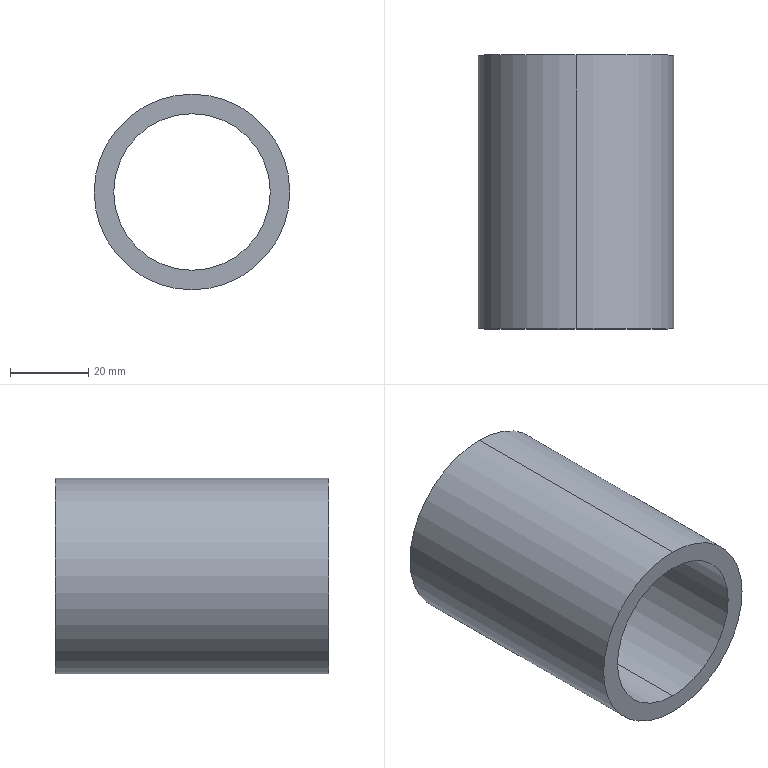Part | STEP file | PN_0036_default | 1 solid | 6 faces | box 50 x 70 x 50 mm | volume 49480 mm3 | cylinder 4 | plane 2 | commonest cylinder face diameters 40 x2 50 x2
STEP:
#1=CARTESIAN_POINT('',(0.,0.,0.));
#2=DIRECTION('',(0.,0.,1.));
#3=DIRECTION('',(1.,0.,0.));
#4=AXIS2_PLACEMENT_3D('',#1,#2,#3);
#5=CARTESIAN_POINT('',(0.,30.,-20.));
#6=VERTEX_POINT('',#5);
#7=CARTESIAN_POINT('',(0.,-40.,-20.));
#8=VERTEX_POINT('',#7);
#9=CARTESIAN_POINT('',(0.,30.,-20.));
#10=DIRECTION('',(0.,-1.,0.));
#11=VECTOR('',#10,1.);
#12=LINE('',#9,#11);
#13=CARTESIAN_POINT('',(0.,30.,0.));
#14=DIRECTION('',(0.,-1.,0.));
#15=DIRECTION('',(0.,0.,-1.));
#16=AXIS2_PLACEMENT_3D('',#13,#14,#15);
#17=CYLINDRICAL_SURFACE('',#16,20.);
#18=CARTESIAN_POINT('',(6.283,0.));
#19=DIRECTION('',(0.,1.));
#20=VECTOR('',#19,1.);
#21=LINE('',#18,#20);
#22=(GEOMETRIC_REPRESENTATION_CONTEXT(2)PARAMETRIC_REPRESENTATION_CONTEXT()REPRESENTATION_CONTEXT('',''));
#23=DEFINITIONAL_REPRESENTATION('',(#21),#22);
#24=PCURVE('',#17,#23);
#25=CARTESIAN_POINT('',(0.,30.,0.));
#26=DIRECTION('',(0.,-1.,0.));
#27=DIRECTION('',(0.,0.,-1.));
#28=AXIS2_PLACEMENT_3D('',#25,#26,#27);
#29=CYLINDRICAL_SURFACE('',#28,20.);
#30=CARTESIAN_POINT('',(0.,0.));
#31=DIRECTION('',(0.,1.));
#32=VECTOR('',#31,1.);
#33=LINE('',#30,#32);
#34=(GEOMETRIC_REPRESENTATION_CONTEXT(2)PARAMETRIC_REPRESENTATION_CONTEXT()REPRESENTATION_CONTEXT('',''));
#35=DEFINITIONAL_REPRESENTATION('',(#33),#34);
#36=PCURVE('',#29,#35);
#37=SURFACE_CURVE('',#12,(#24,#36),.PCURVE_S1.);
#38=EDGE_CURVE('',#6,#8,#37,.T.);
#39=ORIENTED_EDGE('',*,*,#38,.T.);
#40=CARTESIAN_POINT('',(0.,-40.,20.));
#41=VERTEX_POINT('',#40);
#42=CARTESIAN_POINT('',(0.,-40.,0.));
#43=DIRECTION('',(0.,-1.,0.));
#44=DIRECTION('',(0.,0.,-1.));
#45=AXIS2_PLACEMENT_3D('',#42,#43,#44);
#46=CIRCLE('',#45,20.);
#47=CARTESIAN_POINT('',(0.,70.));
#48=DIRECTION('',(1.,0.));
#49=VECTOR('',#48,1.);
#50=LINE('',#47,#49);
#51=(GEOMETRIC_REPRESENTATION_CONTEXT(2)PARAMETRIC_REPRESENTATION_CONTEXT()REPRESENTATION_CONTEXT('',''));
#52=DEFINITIONAL_REPRESENTATION('',(#50),#51);
#53=PCURVE('',#17,#52);
#54=CARTESIAN_POINT('',(20.,-40.,0.));
#55=DIRECTION('',(0.,-1.,0.));
#56=DIRECTION('',(0.,0.,-1.));
#57=AXIS2_PLACEMENT_3D('',#54,#55,#56);
#58=PLANE('',#57);
#59=CARTESIAN_POINT('',(0.,-20.));
#60=DIRECTION('',(1.,0.));
#61=AXIS2_PLACEMENT_2D('',#59,#60);
#62=CIRCLE('',#61,20.);
#63=(GEOMETRIC_REPRESENTATION_CONTEXT(2)PARAMETRIC_REPRESENTATION_CONTEXT()REPRESENTATION_CONTEXT('',''));
#64=DEFINITIONAL_REPRESENTATION('',(#62),#63);
#65=PCURVE('',#58,#64);
#66=SURFACE_CURVE('',#46,(#53,#65),.PCURVE_S1.);
#67=EDGE_CURVE('',#41,#8,#66,.T.);
#68=ORIENTED_EDGE('',*,*,#67,.F.);
#69=CARTESIAN_POINT('',(0.,30.,20.));
#70=VERTEX_POINT('',#69);
#71=CARTESIAN_POINT('',(0.,30.,20.));
#72=DIRECTION('',(0.,-1.,0.));
#73=VECTOR('',#72,1.);
#74=LINE('',#71,#73);
#75=CARTESIAN_POINT('',(3.142,0.));
#76=DIRECTION('',(0.,1.));
#77=VECTOR('',#76,1.);
#78=LINE('',#75,#77);
#79=(GEOMETRIC_REPRESENTATION_CONTEXT(2)PARAMETRIC_REPRESENTATION_CONTEXT()REPRESENTATION_CONTEXT('',''));
#80=DEFINITIONAL_REPRESENTATION('',(#78),#79);
#81=PCURVE('',#17,#80);
#82=CARTESIAN_POINT('',(3.142,0.));
#83=DIRECTION('',(0.,1.));
#84=VECTOR('',#83,1.);
#85=LINE('',#82,#84);
#86=(GEOMETRIC_REPRESENTATION_CONTEXT(2)PARAMETRIC_REPRESENTATION_CONTEXT()REPRESENTATION_CONTEXT('',''));
#87=DEFINITIONAL_REPRESENTATION('',(#85),#86);
#88=PCURVE('',#29,#87);
#89=SURFACE_CURVE('',#74,(#81,#88),.PCURVE_S1.);
#90=EDGE_CURVE('',#70,#41,#89,.T.);
#91=ORIENTED_EDGE('',*,*,#90,.F.);
#92=CARTESIAN_POINT('',(0.,30.,0.));
#93=DIRECTION('',(0.,-1.,0.));
#94=DIRECTION('',(0.,0.,-1.));
#95=AXIS2_PLACEMENT_3D('',#92,#93,#94);
#96=CIRCLE('',#95,20.);
#97=CARTESIAN_POINT('',(0.,0.));
#98=DIRECTION('',(1.,0.));
#99=VECTOR('',#98,1.);
#100=LINE('',#97,#99);
#101=(GEOMETRIC_REPRESENTATION_CONTEXT(2)PARAMETRIC_REPRESENTATION_CONTEXT()REPRESENTATION_CONTEXT('',''));
#102=DEFINITIONAL_REPRESENTATION('',(#100),#101);
#103=PCURVE('',#17,#102);
#104=CARTESIAN_POINT('',(25.,30.,0.));
#105=DIRECTION('',(0.,1.,0.));
#106=DIRECTION('',(0.,0.,1.));
#107=AXIS2_PLACEMENT_3D('',#104,#105,#106);
#108=PLANE('',#107);
#109=CARTESIAN_POINT('',(-20.,-25.));
#110=CARTESIAN_POINT('',(-20.,9.641));
#111=CARTESIAN_POINT('',(10.,-7.679));
#112=CARTESIAN_POINT('',(40.,-25.));
#113=CARTESIAN_POINT('',(10.,-42.321));
#114=CARTESIAN_POINT('',(-20.,-59.641));
#115=CARTESIAN_POINT('',(-20.,-25.));
#116=(BOUNDED_CURVE()B_SPLINE_CURVE(2,(#109,#110,#111,#112,#113,#114,#115),.UNSPECIFIED.,.T.,.F.)B_SPLINE_CURVE_WITH_KNOTS((1,2,2,2,2,1),(-2.094,0.,2.094,4.189,6.283,8.378),.UNSPECIFIED.)CURVE()GEOMETRIC_REPRESENTATION_ITEM()RATIONAL_B_SPLINE_CURVE((1.,0.5,1.,0.5,1.,0.5,1.))REPRESENTATION_ITEM(''));
#117=(GEOMETRIC_REPRESENTATION_CONTEXT(2)PARAMETRIC_REPRESENTATION_CONTEXT()REPRESENTATION_CONTEXT('',''));
#118=DEFINITIONAL_REPRESENTATION('',(#116),#117);
#119=PCURVE('',#108,#118);
#120=SURFACE_CURVE('',#96,(#103,#119),.PCURVE_S1.);
#121=EDGE_CURVE('',#70,#6,#120,.T.);
#122=ORIENTED_EDGE('',*,*,#121,.T.);
#123=EDGE_LOOP('',(#39,#68,#91,#122));
#124=FACE_BOUND('',#123,.F.);
#125=ADVANCED_FACE('',(#124),#17,.F.);
#126=CARTESIAN_POINT('',(0.,30.,-25.));
#127=VERTEX_POINT('',#126);
#128=CARTESIAN_POINT('',(0.,30.,25.));
#129=VERTEX_POINT('',#128);
#130=CARTESIAN_POINT('',(0.,30.,0.));
#131=DIRECTION('',(0.,-1.,0.));
#132=DIRECTION('',(0.,0.,-1.));
#133=AXIS2_PLACEMENT_3D('',#130,#131,#132);
#134=CIRCLE('',#133,25.);
#135=CARTESIAN_POINT('',(0.,30.,0.));
#136=DIRECTION('',(0.,-1.,0.));
#137=DIRECTION('',(0.,0.,-1.));
#138=AXIS2_PLACEMENT_3D('',#135,#136,#137);
#139=CYLINDRICAL_SURFACE('',#138,25.);
#140=CARTESIAN_POINT('',(0.,0.));
#141=DIRECTION('',(1.,0.));
#142=VECTOR('',#141,1.);
#143=LINE('',#140,#142);
#144=(GEOMETRIC_REPRESENTATION_CONTEXT(2)PARAMETRIC_REPRESENTATION_CONTEXT()REPRESENTATION_CONTEXT('',''));
#145=DEFINITIONAL_REPRESENTATION('',(#143),#144);
#146=PCURVE('',#139,#145);
#147=CARTESIAN_POINT('',(-25.,-25.));
#148=CARTESIAN_POINT('',(-25.,18.301));
#149=CARTESIAN_POINT('',(12.5,-3.349));
#150=CARTESIAN_POINT('',(50.,-25.));
#151=CARTESIAN_POINT('',(12.5,-46.651));
#152=CARTESIAN_POINT('',(-25.,-68.301));
#153=CARTESIAN_POINT('',(-25.,-25.));
#154=(BOUNDED_CURVE()B_SPLINE_CURVE(2,(#147,#148,#149,#150,#151,#152,#153),.UNSPECIFIED.,.T.,.F.)B_SPLINE_CURVE_WITH_KNOTS((1,2,2,2,2,1),(-2.094,0.,2.094,4.189,6.283,8.378),.UNSPECIFIED.)CURVE()GEOMETRIC_REPRESENTATION_ITEM()RATIONAL_B_SPLINE_CURVE((1.,0.5,1.,0.5,1.,0.5,1.))REPRESENTATION_ITEM(''));
#155=(GEOMETRIC_REPRESENTATION_CONTEXT(2)PARAMETRIC_REPRESENTATION_CONTEXT()REPRESENTATION_CONTEXT('',''));
#156=DEFINITIONAL_REPRESENTATION('',(#154),#155);
#157=PCURVE('',#108,#156);
#158=SURFACE_CURVE('',#134,(#146,#157),.PCURVE_S1.);
#159=EDGE_CURVE('',#127,#129,#158,.T.);
#160=ORIENTED_EDGE('',*,*,#159,.T.);
#161=CARTESIAN_POINT('',(0.,-40.,25.));
#162=VERTEX_POINT('',#161);
#163=CARTESIAN_POINT('',(0.,30.,25.));
#164=DIRECTION('',(0.,-1.,0.));
#165=VECTOR('',#164,1.);
#166=LINE('',#163,#165);
#167=CARTESIAN_POINT('',(3.142,0.));
#168=DIRECTION('',(0.,1.));
#169=VECTOR('',#168,1.);
#170=LINE('',#167,#169);
#171=(GEOMETRIC_REPRESENTATION_CONTEXT(2)PARAMETRIC_REPRESENTATION_CONTEXT()REPRESENTATION_CONTEXT('',''));
#172=DEFINITIONAL_REPRESENTATION('',(#170),#171);
#173=PCURVE('',#139,#172);
#174=CARTESIAN_POINT('',(0.,30.,0.));
#175=DIRECTION('',(0.,-1.,0.));
#176=DIRECTION('',(0.,0.,-1.));
#177=AXIS2_PLACEMENT_3D('',#174,#175,#176);
#178=CYLINDRICAL_SURFACE('',#177,25.);
#179=CARTESIAN_POINT('',(3.142,0.));
#180=DIRECTION('',(0.,1.));
#181=VECTOR('',#180,1.);
#182=LINE('',#179,#181);
#183=(GEOMETRIC_REPRESENTATION_CONTEXT(2)PARAMETRIC_REPRESENTATION_CONTEXT()REPRESENTATION_CONTEXT('',''));
#184=DEFINITIONAL_REPRESENTATION('',(#182),#183);
#185=PCURVE('',#178,#184);
#186=SURFACE_CURVE('',#166,(#173,#185),.PCURVE_S1.);
#187=EDGE_CURVE('',#129,#162,#186,.T.);
#188=ORIENTED_EDGE('',*,*,#187,.T.);
#189=CARTESIAN_POINT('',(0.,-40.,-25.));
#190=VERTEX_POINT('',#189);
#191=CARTESIAN_POINT('',(0.,-40.,0.));
#192=DIRECTION('',(0.,-1.,0.));
#193=DIRECTION('',(0.,0.,-1.));
#194=AXIS2_PLACEMENT_3D('',#191,#192,#193);
#195=CIRCLE('',#194,25.);
#196=CARTESIAN_POINT('',(0.,70.));
#197=DIRECTION('',(1.,0.));
#198=VECTOR('',#197,1.);
#199=LINE('',#196,#198);
#200=(GEOMETRIC_REPRESENTATION_CONTEXT(2)PARAMETRIC_REPRESENTATION_CONTEXT()REPRESENTATION_CONTEXT('',''));
#201=DEFINITIONAL_REPRESENTATION('',(#199),#200);
#202=PCURVE('',#139,#201);
#203=CARTESIAN_POINT('',(0.,-20.));
#204=DIRECTION('',(1.,0.));
#205=AXIS2_PLACEMENT_2D('',#203,#204);
#206=CIRCLE('',#205,25.);
#207=(GEOMETRIC_REPRESENTATION_CONTEXT(2)PARAMETRIC_REPRESENTATION_CONTEXT()REPRESENTATION_CONTEXT('',''));
#208=DEFINITIONAL_REPRESENTATION('',(#206),#207);
#209=PCURVE('',#58,#208);
#210=SURFACE_CURVE('',#195,(#202,#209),.PCURVE_S1.);
#211=EDGE_CURVE('',#190,#162,#210,.T.);
#212=ORIENTED_EDGE('',*,*,#211,.F.);
#213=CARTESIAN_POINT('',(0.,30.,-25.));
#214=DIRECTION('',(0.,-1.,0.));
#215=VECTOR('',#214,1.);
#216=LINE('',#213,#215);
#217=CARTESIAN_POINT('',(0.,0.));
#218=DIRECTION('',(0.,1.));
#219=VECTOR('',#218,1.);
#220=LINE('',#217,#219);
#221=(GEOMETRIC_REPRESENTATION_CONTEXT(2)PARAMETRIC_REPRESENTATION_CONTEXT()REPRESENTATION_CONTEXT('',''));
#222=DEFINITIONAL_REPRESENTATION('',(#220),#221);
#223=PCURVE('',#139,#222);
#224=CARTESIAN_POINT('',(6.283,0.));
#225=DIRECTION('',(0.,1.));
#226=VECTOR('',#225,1.);
#227=LINE('',#224,#226);
#228=(GEOMETRIC_REPRESENTATION_CONTEXT(2)PARAMETRIC_REPRESENTATION_CONTEXT()REPRESENTATION_CONTEXT('',''));
#229=DEFINITIONAL_REPRESENTATION('',(#227),#228);
#230=PCURVE('',#178,#229);
#231=SURFACE_CURVE('',#216,(#223,#230),.PCURVE_S1.);
#232=EDGE_CURVE('',#127,#190,#231,.T.);
#233=ORIENTED_EDGE('',*,*,#232,.F.);
#234=EDGE_LOOP('',(#160,#188,#212,#233));
#235=FACE_BOUND('',#234,.T.);
#236=ADVANCED_FACE('',(#235),#139,.T.);
#237=ORIENTED_EDGE('',*,*,#211,.T.);
#238=CARTESIAN_POINT('',(0.,-40.,0.));
#239=DIRECTION('',(0.,-1.,0.));
#240=DIRECTION('',(0.,0.,-1.));
#241=AXIS2_PLACEMENT_3D('',#238,#239,#240);
#242=CIRCLE('',#241,25.);
#243=CARTESIAN_POINT('',(0.,-20.));
#244=DIRECTION('',(1.,0.));
#245=AXIS2_PLACEMENT_2D('',#243,#244);
#246=CIRCLE('',#245,25.);
#247=(GEOMETRIC_REPRESENTATION_CONTEXT(2)PARAMETRIC_REPRESENTATION_CONTEXT()REPRESENTATION_CONTEXT('',''));
#248=DEFINITIONAL_REPRESENTATION('',(#246),#247);
#249=PCURVE('',#58,#248);
#250=CARTESIAN_POINT('',(0.,70.));
#251=DIRECTION('',(1.,0.));
#252=VECTOR('',#251,1.);
#253=LINE('',#250,#252);
#254=(GEOMETRIC_REPRESENTATION_CONTEXT(2)PARAMETRIC_REPRESENTATION_CONTEXT()REPRESENTATION_CONTEXT('',''));
#255=DEFINITIONAL_REPRESENTATION('',(#253),#254);
#256=PCURVE('',#178,#255);
#257=SURFACE_CURVE('',#242,(#249,#256),.PCURVE_S1.);
#258=EDGE_CURVE('',#162,#190,#257,.T.);
#259=ORIENTED_EDGE('',*,*,#258,.T.);
#260=EDGE_LOOP('',(#237,#259));
#261=FACE_BOUND('',#260,.T.);
#262=CARTESIAN_POINT('',(0.,-40.,0.));
#263=DIRECTION('',(0.,-1.,0.));
#264=DIRECTION('',(0.,0.,-1.));
#265=AXIS2_PLACEMENT_3D('',#262,#263,#264);
#266=CIRCLE('',#265,20.);
#267=CARTESIAN_POINT('',(0.,-20.));
#268=DIRECTION('',(1.,0.));
#269=AXIS2_PLACEMENT_2D('',#267,#268);
#270=CIRCLE('',#269,20.);
#271=(GEOMETRIC_REPRESENTATION_CONTEXT(2)PARAMETRIC_REPRESENTATION_CONTEXT()REPRESENTATION_CONTEXT('',''));
#272=DEFINITIONAL_REPRESENTATION('',(#270),#271);
#273=PCURVE('',#58,#272);
#274=CARTESIAN_POINT('',(0.,70.));
#275=DIRECTION('',(1.,0.));
#276=VECTOR('',#275,1.);
#277=LINE('',#274,#276);
#278=(GEOMETRIC_REPRESENTATION_CONTEXT(2)PARAMETRIC_REPRESENTATION_CONTEXT()REPRESENTATION_CONTEXT('',''));
#279=DEFINITIONAL_REPRESENTATION('',(#277),#278);
#280=PCURVE('',#29,#279);
#281=SURFACE_CURVE('',#266,(#273,#280),.PCURVE_S1.);
#282=EDGE_CURVE('',#8,#41,#281,.T.);
#283=ORIENTED_EDGE('',*,*,#282,.F.);
#284=ORIENTED_EDGE('',*,*,#67,.F.);
#285=EDGE_LOOP('',(#283,#284));
#286=FACE_BOUND('',#285,.T.);
#287=ADVANCED_FACE('',(#261,#286),#58,.T.);
#288=ORIENTED_EDGE('',*,*,#187,.F.);
#289=CARTESIAN_POINT('',(0.,30.,0.));
#290=DIRECTION('',(0.,-1.,0.));
#291=DIRECTION('',(0.,0.,-1.));
#292=AXIS2_PLACEMENT_3D('',#289,#290,#291);
#293=CIRCLE('',#292,25.);
#294=CARTESIAN_POINT('',(0.,0.));
#295=DIRECTION('',(1.,0.));
#296=VECTOR('',#295,1.);
#297=LINE('',#294,#296);
#298=(GEOMETRIC_REPRESENTATION_CONTEXT(2)PARAMETRIC_REPRESENTATION_CONTEXT()REPRESENTATION_CONTEXT('',''));
#299=DEFINITIONAL_REPRESENTATION('',(#297),#298);
#300=PCURVE('',#178,#299);
#301=CARTESIAN_POINT('',(-25.,-25.));
#302=CARTESIAN_POINT('',(-25.,18.301));
#303=CARTESIAN_POINT('',(12.5,-3.349));
#304=CARTESIAN_POINT('',(50.,-25.));
#305=CARTESIAN_POINT('',(12.5,-46.651));
#306=CARTESIAN_POINT('',(-25.,-68.301));
#307=CARTESIAN_POINT('',(-25.,-25.));
#308=(BOUNDED_CURVE()B_SPLINE_CURVE(2,(#301,#302,#303,#304,#305,#306,#307),.UNSPECIFIED.,.T.,.F.)B_SPLINE_CURVE_WITH_KNOTS((1,2,2,2,2,1),(-2.094,0.,2.094,4.189,6.283,8.378),.UNSPECIFIED.)CURVE()GEOMETRIC_REPRESENTATION_ITEM()RATIONAL_B_SPLINE_CURVE((1.,0.5,1.,0.5,1.,0.5,1.))REPRESENTATION_ITEM(''));
#309=(GEOMETRIC_REPRESENTATION_CONTEXT(2)PARAMETRIC_REPRESENTATION_CONTEXT()REPRESENTATION_CONTEXT('',''));
#310=DEFINITIONAL_REPRESENTATION('',(#308),#309);
#311=PCURVE('',#108,#310);
#312=SURFACE_CURVE('',#293,(#300,#311),.PCURVE_S1.);
#313=EDGE_CURVE('',#129,#127,#312,.T.);
#314=ORIENTED_EDGE('',*,*,#313,.T.);
#315=ORIENTED_EDGE('',*,*,#232,.T.);
#316=ORIENTED_EDGE('',*,*,#258,.F.);
#317=EDGE_LOOP('',(#288,#314,#315,#316));
#318=FACE_BOUND('',#317,.T.);
#319=ADVANCED_FACE('',(#318),#178,.T.);
#320=CARTESIAN_POINT('',(0.,30.,0.));
#321=DIRECTION('',(0.,-1.,0.));
#322=DIRECTION('',(0.,0.,-1.));
#323=AXIS2_PLACEMENT_3D('',#320,#321,#322);
#324=CIRCLE('',#323,20.);
#325=CARTESIAN_POINT('',(-20.,-25.));
#326=CARTESIAN_POINT('',(-20.,9.641));
#327=CARTESIAN_POINT('',(10.,-7.679));
#328=CARTESIAN_POINT('',(40.,-25.));
#329=CARTESIAN_POINT('',(10.,-42.321));
#330=CARTESIAN_POINT('',(-20.,-59.641));
#331=CARTESIAN_POINT('',(-20.,-25.));
#332=(BOUNDED_CURVE()B_SPLINE_CURVE(2,(#325,#326,#327,#328,#329,#330,#331),.UNSPECIFIED.,.T.,.F.)B_SPLINE_CURVE_WITH_KNOTS((1,2,2,2,2,1),(-2.094,0.,2.094,4.189,6.283,8.378),.UNSPECIFIED.)CURVE()GEOMETRIC_REPRESENTATION_ITEM()RATIONAL_B_SPLINE_CURVE((1.,0.5,1.,0.5,1.,0.5,1.))REPRESENTATION_ITEM(''));
#333=(GEOMETRIC_REPRESENTATION_CONTEXT(2)PARAMETRIC_REPRESENTATION_CONTEXT()REPRESENTATION_CONTEXT('',''));
#334=DEFINITIONAL_REPRESENTATION('',(#332),#333);
#335=PCURVE('',#108,#334);
#336=CARTESIAN_POINT('',(0.,0.));
#337=DIRECTION('',(1.,0.));
#338=VECTOR('',#337,1.);
#339=LINE('',#336,#338);
#340=(GEOMETRIC_REPRESENTATION_CONTEXT(2)PARAMETRIC_REPRESENTATION_CONTEXT()REPRESENTATION_CONTEXT('',''));
#341=DEFINITIONAL_REPRESENTATION('',(#339),#340);
#342=PCURVE('',#29,#341);
#343=SURFACE_CURVE('',#324,(#335,#342),.PCURVE_S1.);
#344=EDGE_CURVE('',#6,#70,#343,.T.);
#345=ORIENTED_EDGE('',*,*,#344,.T.);
#346=ORIENTED_EDGE('',*,*,#121,.T.);
#347=EDGE_LOOP('',(#345,#346));
#348=FACE_BOUND('',#347,.T.);
#349=ORIENTED_EDGE('',*,*,#159,.F.);
#350=ORIENTED_EDGE('',*,*,#313,.F.);
#351=EDGE_LOOP('',(#349,#350));
#352=FACE_BOUND('',#351,.T.);
#353=ADVANCED_FACE('',(#348,#352),#108,.T.);
#354=ORIENTED_EDGE('',*,*,#282,.F.);
#355=ORIENTED_EDGE('',*,*,#38,.F.);
#356=ORIENTED_EDGE('',*,*,#344,.T.);
#357=ORIENTED_EDGE('',*,*,#90,.T.);
#358=EDGE_LOOP('',(#354,#355,#356,#357));
#359=FACE_BOUND('',#358,.F.);
#360=ADVANCED_FACE('',(#359),#29,.F.);
#361=CLOSED_SHELL('',(#125,#236,#287,#319,#353,#360));
#362=MANIFOLD_SOLID_BREP('',#361);
#363=(LENGTH_UNIT()NAMED_UNIT(*)SI_UNIT(.MILLI.,.METRE.));
#364=UNCERTAINTY_MEASURE_WITH_UNIT(LENGTH_MEASURE(0.0000001),#363,'','');
#365=(NAMED_UNIT(*)PLANE_ANGLE_UNIT()SI_UNIT($,.RADIAN.));
#366=(NAMED_UNIT(*)SI_UNIT($,.STERADIAN.)SOLID_ANGLE_UNIT());
#367=(GEOMETRIC_REPRESENTATION_CONTEXT(3)GLOBAL_UNCERTAINTY_ASSIGNED_CONTEXT((#364))GLOBAL_UNIT_ASSIGNED_CONTEXT((#363,#365,#366))REPRESENTATION_CONTEXT('',''));
#368=ADVANCED_BREP_SHAPE_REPRESENTATION('',(#4,#362),#367);